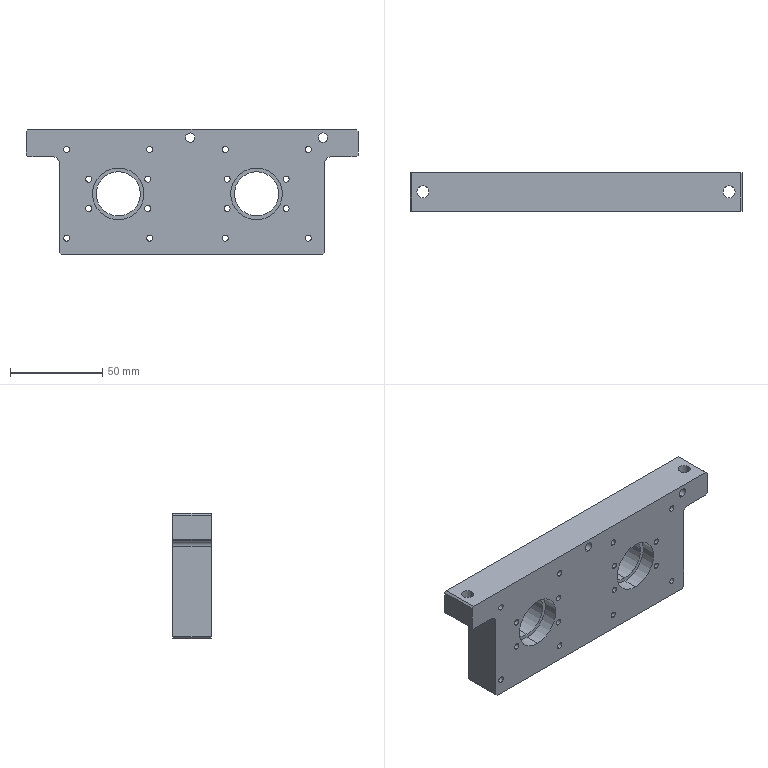Part | STEP file | Bearing fixing plate | 1 solid | 68 faces | box 180 x 21 x 68 mm | volume 190682 mm3 | cylinder 50 | plane 18 | commonest cylinder face diameters 3.3 x32 5 x4 6.5 x4 24 x4 28 x4 6 x2